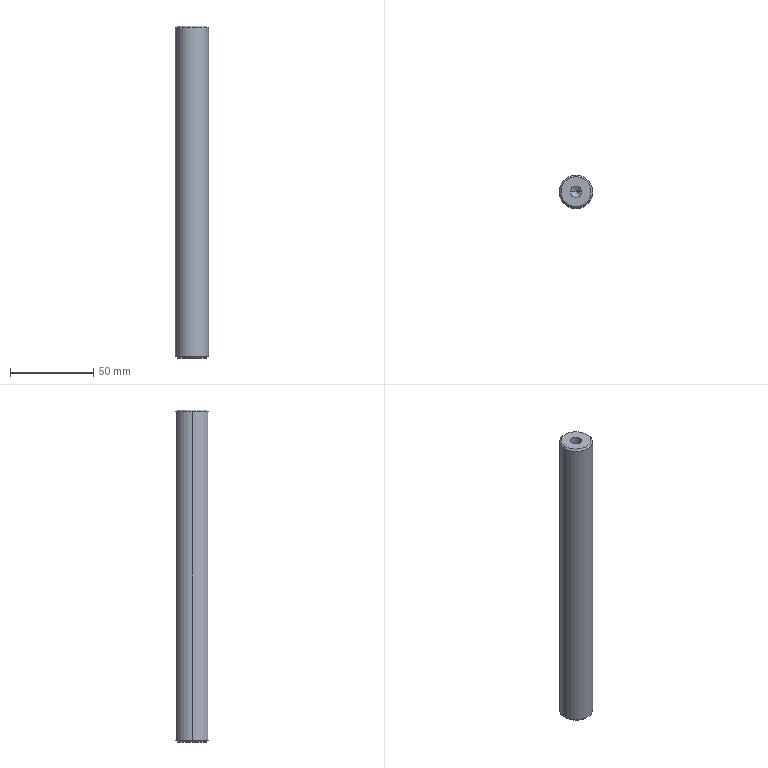Part | SolidWorks | features HoleWzd 2, Chamfer 1, Extrusion 1 | 1 solid | 16 faces | box 20 x 20 x 200 mm | volume 61287 mm3 | cone 8 | cylinder 6 | plane 2 | commonest cylinder face diameters 6.8 x4 20 x2
STEP:
#1=CARTESIAN_POINT('',(9.,0.,200.));
#2=VERTEX_POINT('',#1);
#3=CARTESIAN_POINT('',(-9.,0.,200.));
#4=VERTEX_POINT('',#3);
#5=CARTESIAN_POINT('',(0.,0.,200.));
#6=DIRECTION('',(0.,0.,1.));
#7=DIRECTION('',(1.,0.,0.));
#8=AXIS2_PLACEMENT_3D('',#5,#6,#7);
#9=CIRCLE('',#8,9.);
#10=EDGE_CURVE('',#2,#4,#9,.T.);
#11=ORIENTED_EDGE('',*,*,#10,.F.);
#12=CARTESIAN_POINT('',(10.,0.,199.));
#13=VERTEX_POINT('',#12);
#14=CARTESIAN_POINT('',(9.,0.,200.));
#15=DIRECTION('',(0.7071,0.,-0.7071));
#16=VECTOR('',#15,1000.);
#17=LINE('',#14,#16);
#18=EDGE_CURVE('',#2,#13,#17,.T.);
#19=ORIENTED_EDGE('',*,*,#18,.T.);
#20=CARTESIAN_POINT('',(-10.,0.,199.));
#21=VERTEX_POINT('',#20);
#22=CARTESIAN_POINT('',(0.,0.,199.));
#23=DIRECTION('',(0.,0.,-1.));
#24=DIRECTION('',(1.,0.,0.));
#25=AXIS2_PLACEMENT_3D('',#22,#23,#24);
#26=CIRCLE('',#25,10.);
#27=EDGE_CURVE('',#21,#13,#26,.T.);
#28=ORIENTED_EDGE('',*,*,#27,.F.);
#29=CARTESIAN_POINT('',(-9.,0.,200.));
#30=DIRECTION('',(-0.7071,0.,-0.7071));
#31=VECTOR('',#30,1000.);
#32=LINE('',#29,#31);
#33=EDGE_CURVE('',#4,#21,#32,.T.);
#34=ORIENTED_EDGE('',*,*,#33,.F.);
#35=EDGE_LOOP('',(#11,#19,#28,#34));
#36=FACE_OUTER_BOUND('',#35,.T.);
#37=CARTESIAN_POINT('',(0.,0.,200.));
#38=DIRECTION('',(0.,0.,-1.));
#39=DIRECTION('',(-1.,0.,0.));
#40=AXIS2_PLACEMENT_3D('',#37,#38,#39);
#41=CONICAL_SURFACE('',#40,9.,0.7854);
#42=ADVANCED_FACE('',(#36),#41,.T.);
#43=CARTESIAN_POINT('',(-9.,0.,0.));
#44=VERTEX_POINT('',#43);
#45=CARTESIAN_POINT('',(9.,0.,0.));
#46=VERTEX_POINT('',#45);
#47=CARTESIAN_POINT('',(0.,0.,0.));
#48=DIRECTION('',(0.,0.,-1.));
#49=DIRECTION('',(1.,0.,0.));
#50=AXIS2_PLACEMENT_3D('',#47,#48,#49);
#51=CIRCLE('',#50,9.);
#52=EDGE_CURVE('',#44,#46,#51,.T.);
#53=ORIENTED_EDGE('',*,*,#52,.F.);
#54=CARTESIAN_POINT('',(-10.,0.,1.));
#55=VERTEX_POINT('',#54);
#56=CARTESIAN_POINT('',(-10.,0.,1.));
#57=DIRECTION('',(-0.7071,0.,0.7071));
#58=VECTOR('',#57,1000.);
#59=LINE('',#56,#58);
#60=EDGE_CURVE('',#44,#55,#59,.T.);
#61=ORIENTED_EDGE('',*,*,#60,.T.);
#62=CARTESIAN_POINT('',(10.,0.,1.));
#63=VERTEX_POINT('',#62);
#64=CARTESIAN_POINT('',(0.,0.,1.));
#65=DIRECTION('',(0.,0.,1.));
#66=DIRECTION('',(1.,0.,0.));
#67=AXIS2_PLACEMENT_3D('',#64,#65,#66);
#68=CIRCLE('',#67,10.);
#69=EDGE_CURVE('',#63,#55,#68,.T.);
#70=ORIENTED_EDGE('',*,*,#69,.F.);
#71=CARTESIAN_POINT('',(10.,0.,1.));
#72=DIRECTION('',(0.7071,0.,0.7071));
#73=VECTOR('',#72,1000.);
#74=LINE('',#71,#73);
#75=EDGE_CURVE('',#46,#63,#74,.T.);
#76=ORIENTED_EDGE('',*,*,#75,.F.);
#77=EDGE_LOOP('',(#53,#61,#70,#76));
#78=FACE_OUTER_BOUND('',#77,.T.);
#79=CARTESIAN_POINT('',(0.,0.,1.));
#80=DIRECTION('',(0.,0.,1.));
#81=DIRECTION('',(1.,0.,0.));
#82=AXIS2_PLACEMENT_3D('',#79,#80,#81);
#83=CONICAL_SURFACE('',#82,10.,0.7854);
#84=ADVANCED_FACE('',(#78),#83,.T.);
#85=CARTESIAN_POINT('',(-3.4,0.,180.25));
#86=VERTEX_POINT('',#85);
#87=CARTESIAN_POINT('',(3.4,0.,180.25));
#88=VERTEX_POINT('',#87);
#89=CARTESIAN_POINT('',(0.,0.,180.25));
#90=DIRECTION('',(0.,0.,1.));
#91=DIRECTION('',(1.,0.,0.));
#92=AXIS2_PLACEMENT_3D('',#89,#90,#91);
#93=CIRCLE('',#92,3.4);
#94=EDGE_CURVE('',#86,#88,#93,.T.);
#95=ORIENTED_EDGE('',*,*,#94,.F.);
#96=CARTESIAN_POINT('',(-3.4,0.,200.));
#97=VERTEX_POINT('',#96);
#98=CARTESIAN_POINT('',(-3.4,0.,200.));
#99=DIRECTION('',(0.,0.,1.));
#100=VECTOR('',#99,1000.);
#101=LINE('',#98,#100);
#102=EDGE_CURVE('',#86,#97,#101,.T.);
#103=ORIENTED_EDGE('',*,*,#102,.T.);
#104=CARTESIAN_POINT('',(3.4,0.,200.));
#105=VERTEX_POINT('',#104);
#106=CARTESIAN_POINT('',(0.,0.,200.));
#107=DIRECTION('',(0.,0.,1.));
#108=DIRECTION('',(1.,0.,0.));
#109=AXIS2_PLACEMENT_3D('',#106,#107,#108);
#110=CIRCLE('',#109,3.4);
#111=EDGE_CURVE('',#97,#105,#110,.T.);
#112=ORIENTED_EDGE('',*,*,#111,.T.);
#113=CARTESIAN_POINT('',(3.4,0.,200.));
#114=DIRECTION('',(0.,0.,1.));
#115=VECTOR('',#114,1000.);
#116=LINE('',#113,#115);
#117=EDGE_CURVE('',#88,#105,#116,.T.);
#118=ORIENTED_EDGE('',*,*,#117,.F.);
#119=EDGE_LOOP('',(#95,#103,#112,#118));
#120=FACE_OUTER_BOUND('',#119,.T.);
#121=CARTESIAN_POINT('',(0.,0.,200.));
#122=DIRECTION('',(0.,0.,1.));
#123=DIRECTION('',(1.,0.,0.));
#124=AXIS2_PLACEMENT_3D('',#121,#122,#123);
#125=CYLINDRICAL_SURFACE('',#124,3.4);
#126=ADVANCED_FACE('',(#120),#125,.F.);
#127=CARTESIAN_POINT('',(0.,0.,178.207));
#128=VERTEX_POINT('',#127);
#129=CARTESIAN_POINT('',(3.4,0.,180.25));
#130=DIRECTION('',(0.8572,0.,0.515));
#131=VECTOR('',#130,1000.);
#132=LINE('',#129,#131);
#133=EDGE_CURVE('',#128,#88,#132,.T.);
#134=ORIENTED_EDGE('',*,*,#133,.F.);
#135=CARTESIAN_POINT('',(-3.4,0.,180.25));
#136=DIRECTION('',(-0.8572,0.,0.515));
#137=VECTOR('',#136,1000.);
#138=LINE('',#135,#137);
#139=EDGE_CURVE('',#128,#86,#138,.T.);
#140=ORIENTED_EDGE('',*,*,#139,.T.);
#141=ORIENTED_EDGE('',*,*,#94,.T.);
#142=EDGE_LOOP('',(#134,#140,#141));
#143=FACE_OUTER_BOUND('',#142,.T.);
#144=CARTESIAN_POINT('',(0.,0.,180.25));
#145=DIRECTION('',(0.,0.,1.));
#146=DIRECTION('',(1.,0.,0.));
#147=AXIS2_PLACEMENT_3D('',#144,#145,#146);
#148=CONICAL_SURFACE('',#147,3.4,1.03);
#149=ADVANCED_FACE('',(#143),#148,.F.);
#150=CARTESIAN_POINT('',(3.4,0.,19.75));
#151=VERTEX_POINT('',#150);
#152=CARTESIAN_POINT('',(-3.4,0.,19.75));
#153=VERTEX_POINT('',#152);
#154=CARTESIAN_POINT('',(0.,0.,19.75));
#155=DIRECTION('',(0.,0.,-1.));
#156=DIRECTION('',(-1.,0.,0.));
#157=AXIS2_PLACEMENT_3D('',#154,#155,#156);
#158=CIRCLE('',#157,3.4);
#159=EDGE_CURVE('',#151,#153,#158,.T.);
#160=ORIENTED_EDGE('',*,*,#159,.F.);
#161=CARTESIAN_POINT('',(3.4,0.,0.));
#162=VERTEX_POINT('',#161);
#163=CARTESIAN_POINT('',(3.4,0.,0.));
#164=DIRECTION('',(0.,0.,-1.));
#165=VECTOR('',#164,1000.);
#166=LINE('',#163,#165);
#167=EDGE_CURVE('',#151,#162,#166,.T.);
#168=ORIENTED_EDGE('',*,*,#167,.T.);
#169=CARTESIAN_POINT('',(-3.4,0.,0.));
#170=VERTEX_POINT('',#169);
#171=CARTESIAN_POINT('',(0.,0.,0.));
#172=DIRECTION('',(0.,0.,-1.));
#173=DIRECTION('',(-1.,0.,0.));
#174=AXIS2_PLACEMENT_3D('',#171,#172,#173);
#175=CIRCLE('',#174,3.4);
#176=EDGE_CURVE('',#162,#170,#175,.T.);
#177=ORIENTED_EDGE('',*,*,#176,.T.);
#178=CARTESIAN_POINT('',(-3.4,0.,0.));
#179=DIRECTION('',(0.,0.,-1.));
#180=VECTOR('',#179,1000.);
#181=LINE('',#178,#180);
#182=EDGE_CURVE('',#153,#170,#181,.T.);
#183=ORIENTED_EDGE('',*,*,#182,.F.);
#184=EDGE_LOOP('',(#160,#168,#177,#183));
#185=FACE_OUTER_BOUND('',#184,.T.);
#186=CARTESIAN_POINT('',(0.,0.,0.));
#187=DIRECTION('',(0.,0.,-1.));
#188=DIRECTION('',(-1.,0.,0.));
#189=AXIS2_PLACEMENT_3D('',#186,#187,#188);
#190=CYLINDRICAL_SURFACE('',#189,3.4);
#191=ADVANCED_FACE('',(#185),#190,.F.);
#192=CARTESIAN_POINT('',(0.,0.,21.793));
#193=VERTEX_POINT('',#192);
#194=CARTESIAN_POINT('',(-3.4,0.,19.75));
#195=DIRECTION('',(-0.8572,0.,-0.515));
#196=VECTOR('',#195,1000.);
#197=LINE('',#194,#196);
#198=EDGE_CURVE('',#193,#153,#197,.T.);
#199=ORIENTED_EDGE('',*,*,#198,.F.);
#200=CARTESIAN_POINT('',(3.4,0.,19.75));
#201=DIRECTION('',(0.8572,0.,-0.515));
#202=VECTOR('',#201,1000.);
#203=LINE('',#200,#202);
#204=EDGE_CURVE('',#193,#151,#203,.T.);
#205=ORIENTED_EDGE('',*,*,#204,.T.);
#206=ORIENTED_EDGE('',*,*,#159,.T.);
#207=EDGE_LOOP('',(#199,#205,#206));
#208=FACE_OUTER_BOUND('',#207,.T.);
#209=CARTESIAN_POINT('',(0.,0.,19.75));
#210=DIRECTION('',(0.,0.,-1.));
#211=DIRECTION('',(-1.,0.,0.));
#212=AXIS2_PLACEMENT_3D('',#209,#210,#211);
#213=CONICAL_SURFACE('',#212,3.4,1.03);
#214=ADVANCED_FACE('',(#208),#213,.F.);
#215=ORIENTED_EDGE('',*,*,#27,.T.);
#216=CARTESIAN_POINT('',(10.,0.,200.));
#217=DIRECTION('',(0.,0.,-1.));
#218=VECTOR('',#217,1000.);
#219=LINE('',#216,#218);
#220=EDGE_CURVE('',#13,#63,#219,.T.);
#221=ORIENTED_EDGE('',*,*,#220,.T.);
#222=ORIENTED_EDGE('',*,*,#69,.T.);
#223=CARTESIAN_POINT('',(-10.,0.,200.));
#224=DIRECTION('',(0.,0.,-1.));
#225=VECTOR('',#224,1000.);
#226=LINE('',#223,#225);
#227=EDGE_CURVE('',#21,#55,#226,.T.);
#228=ORIENTED_EDGE('',*,*,#227,.F.);
#229=EDGE_LOOP('',(#215,#221,#222,#228));
#230=FACE_OUTER_BOUND('',#229,.T.);
#231=CARTESIAN_POINT('',(0.,0.,200.));
#232=DIRECTION('',(0.,0.,-1.));
#233=DIRECTION('',(-1.,0.,0.));
#234=AXIS2_PLACEMENT_3D('',#231,#232,#233);
#235=CYLINDRICAL_SURFACE('',#234,10.);
#236=ADVANCED_FACE('',(#230),#235,.T.);
#237=ORIENTED_EDGE('',*,*,#220,.F.);
#238=CARTESIAN_POINT('',(0.,0.,199.));
#239=DIRECTION('',(0.,0.,-1.));
#240=DIRECTION('',(1.,0.,0.));
#241=AXIS2_PLACEMENT_3D('',#238,#239,#240);
#242=CIRCLE('',#241,10.);
#243=EDGE_CURVE('',#13,#21,#242,.T.);
#244=ORIENTED_EDGE('',*,*,#243,.T.);
#245=ORIENTED_EDGE('',*,*,#227,.T.);
#246=CARTESIAN_POINT('',(0.,0.,1.));
#247=DIRECTION('',(0.,0.,1.));
#248=DIRECTION('',(1.,0.,0.));
#249=AXIS2_PLACEMENT_3D('',#246,#247,#248);
#250=CIRCLE('',#249,10.);
#251=EDGE_CURVE('',#55,#63,#250,.T.);
#252=ORIENTED_EDGE('',*,*,#251,.T.);
#253=EDGE_LOOP('',(#237,#244,#245,#252));
#254=FACE_OUTER_BOUND('',#253,.T.);
#255=CARTESIAN_POINT('',(0.,0.,200.));
#256=DIRECTION('',(0.,0.,-1.));
#257=DIRECTION('',(-1.,0.,0.));
#258=AXIS2_PLACEMENT_3D('',#255,#256,#257);
#259=CYLINDRICAL_SURFACE('',#258,10.);
#260=ADVANCED_FACE('',(#254),#259,.T.);
#261=CARTESIAN_POINT('',(0.,0.,200.));
#262=DIRECTION('',(0.,0.,1.));
#263=DIRECTION('',(1.,0.,0.));
#264=AXIS2_PLACEMENT_3D('',#261,#262,#263);
#265=CIRCLE('',#264,9.);
#266=EDGE_CURVE('',#4,#2,#265,.T.);
#267=ORIENTED_EDGE('',*,*,#266,.T.);
#268=ORIENTED_EDGE('',*,*,#10,.T.);
#269=EDGE_LOOP('',(#267,#268));
#270=FACE_OUTER_BOUND('',#269,.T.);
#271=CARTESIAN_POINT('',(0.,0.,200.));
#272=DIRECTION('',(0.,0.,1.));
#273=DIRECTION('',(1.,0.,0.));
#274=AXIS2_PLACEMENT_3D('',#271,#272,#273);
#275=CIRCLE('',#274,3.4);
#276=EDGE_CURVE('',#105,#97,#275,.T.);
#277=ORIENTED_EDGE('',*,*,#276,.F.);
#278=ORIENTED_EDGE('',*,*,#111,.F.);
#279=EDGE_LOOP('',(#277,#278));
#280=FACE_BOUND('',#279,.T.);
#281=CARTESIAN_POINT('',(0.,0.,200.));
#282=DIRECTION('',(0.,0.,1.));
#283=DIRECTION('',(1.,0.,0.));
#284=AXIS2_PLACEMENT_3D('',#281,#282,#283);
#285=PLANE('',#284);
#286=ADVANCED_FACE('',(#270,#280),#285,.T.);
#287=CARTESIAN_POINT('',(0.,0.,0.));
#288=DIRECTION('',(0.,0.,-1.));
#289=DIRECTION('',(1.,0.,0.));
#290=AXIS2_PLACEMENT_3D('',#287,#288,#289);
#291=CIRCLE('',#290,9.);
#292=EDGE_CURVE('',#46,#44,#291,.T.);
#293=ORIENTED_EDGE('',*,*,#292,.T.);
#294=ORIENTED_EDGE('',*,*,#52,.T.);
#295=EDGE_LOOP('',(#293,#294));
#296=FACE_OUTER_BOUND('',#295,.T.);
#297=CARTESIAN_POINT('',(0.,0.,0.));
#298=DIRECTION('',(0.,0.,-1.));
#299=DIRECTION('',(-1.,0.,0.));
#300=AXIS2_PLACEMENT_3D('',#297,#298,#299);
#301=CIRCLE('',#300,3.4);
#302=EDGE_CURVE('',#170,#162,#301,.T.);
#303=ORIENTED_EDGE('',*,*,#302,.F.);
#304=ORIENTED_EDGE('',*,*,#176,.F.);
#305=EDGE_LOOP('',(#303,#304));
#306=FACE_BOUND('',#305,.T.);
#307=CARTESIAN_POINT('',(0.,0.,0.));
#308=DIRECTION('',(0.,0.,1.));
#309=DIRECTION('',(1.,0.,0.));
#310=AXIS2_PLACEMENT_3D('',#307,#308,#309);
#311=PLANE('',#310);
#312=ADVANCED_FACE('',(#296,#306),#311,.F.);
#313=ORIENTED_EDGE('',*,*,#204,.F.);
#314=ORIENTED_EDGE('',*,*,#198,.T.);
#315=CARTESIAN_POINT('',(0.,0.,19.75));
#316=DIRECTION('',(0.,0.,-1.));
#317=DIRECTION('',(-1.,0.,0.));
#318=AXIS2_PLACEMENT_3D('',#315,#316,#317);
#319=CIRCLE('',#318,3.4);
#320=EDGE_CURVE('',#153,#151,#319,.T.);
#321=ORIENTED_EDGE('',*,*,#320,.T.);
#322=EDGE_LOOP('',(#313,#314,#321));
#323=FACE_OUTER_BOUND('',#322,.T.);
#324=CARTESIAN_POINT('',(0.,0.,19.75));
#325=DIRECTION('',(0.,0.,-1.));
#326=DIRECTION('',(-1.,0.,0.));
#327=AXIS2_PLACEMENT_3D('',#324,#325,#326);
#328=CONICAL_SURFACE('',#327,3.4,1.03);
#329=ADVANCED_FACE('',(#323),#328,.F.);
#330=ORIENTED_EDGE('',*,*,#167,.F.);
#331=ORIENTED_EDGE('',*,*,#320,.F.);
#332=ORIENTED_EDGE('',*,*,#182,.T.);
#333=ORIENTED_EDGE('',*,*,#302,.T.);
#334=EDGE_LOOP('',(#330,#331,#332,#333));
#335=FACE_OUTER_BOUND('',#334,.T.);
#336=CARTESIAN_POINT('',(0.,0.,0.));
#337=DIRECTION('',(0.,0.,-1.));
#338=DIRECTION('',(-1.,0.,0.));
#339=AXIS2_PLACEMENT_3D('',#336,#337,#338);
#340=CYLINDRICAL_SURFACE('',#339,3.4);
#341=ADVANCED_FACE('',(#335),#340,.F.);
#342=ORIENTED_EDGE('',*,*,#139,.F.);
#343=ORIENTED_EDGE('',*,*,#133,.T.);
#344=CARTESIAN_POINT('',(0.,0.,180.25));
#345=DIRECTION('',(0.,0.,1.));
#346=DIRECTION('',(1.,0.,0.));
#347=AXIS2_PLACEMENT_3D('',#344,#345,#346);
#348=CIRCLE('',#347,3.4);
#349=EDGE_CURVE('',#88,#86,#348,.T.);
#350=ORIENTED_EDGE('',*,*,#349,.T.);
#351=EDGE_LOOP('',(#342,#343,#350));
#352=FACE_OUTER_BOUND('',#351,.T.);
#353=CARTESIAN_POINT('',(0.,0.,180.25));
#354=DIRECTION('',(0.,0.,1.));
#355=DIRECTION('',(1.,0.,0.));
#356=AXIS2_PLACEMENT_3D('',#353,#354,#355);
#357=CONICAL_SURFACE('',#356,3.4,1.03);
#358=ADVANCED_FACE('',(#352),#357,.F.);
#359=ORIENTED_EDGE('',*,*,#102,.F.);
#360=ORIENTED_EDGE('',*,*,#349,.F.);
#361=ORIENTED_EDGE('',*,*,#117,.T.);
#362=ORIENTED_EDGE('',*,*,#276,.T.);
#363=EDGE_LOOP('',(#359,#360,#361,#362));
#364=FACE_OUTER_BOUND('',#363,.T.);
#365=CARTESIAN_POINT('',(0.,0.,200.));
#366=DIRECTION('',(0.,0.,1.));
#367=DIRECTION('',(1.,0.,0.));
#368=AXIS2_PLACEMENT_3D('',#365,#366,#367);
#369=CYLINDRICAL_SURFACE('',#368,3.4);
#370=ADVANCED_FACE('',(#364),#369,.F.);
#371=ORIENTED_EDGE('',*,*,#60,.F.);
#372=ORIENTED_EDGE('',*,*,#292,.F.);
#373=ORIENTED_EDGE('',*,*,#75,.T.);
#374=ORIENTED_EDGE('',*,*,#251,.F.);
#375=EDGE_LOOP('',(#371,#372,#373,#374));
#376=FACE_OUTER_BOUND('',#375,.T.);
#377=CARTESIAN_POINT('',(0.,0.,1.));
#378=DIRECTION('',(0.,0.,1.));
#379=DIRECTION('',(1.,0.,0.));
#380=AXIS2_PLACEMENT_3D('',#377,#378,#379);
#381=CONICAL_SURFACE('',#380,10.,0.7854);
#382=ADVANCED_FACE('',(#376),#381,.T.);
#383=ORIENTED_EDGE('',*,*,#18,.F.);
#384=ORIENTED_EDGE('',*,*,#266,.F.);
#385=ORIENTED_EDGE('',*,*,#33,.T.);
#386=ORIENTED_EDGE('',*,*,#243,.F.);
#387=EDGE_LOOP('',(#383,#384,#385,#386));
#388=FACE_OUTER_BOUND('',#387,.T.);
#389=CARTESIAN_POINT('',(0.,0.,200.));
#390=DIRECTION('',(0.,0.,-1.));
#391=DIRECTION('',(-1.,0.,0.));
#392=AXIS2_PLACEMENT_3D('',#389,#390,#391);
#393=CONICAL_SURFACE('',#392,9.,0.7854);
#394=ADVANCED_FACE('',(#388),#393,.T.);
#395=CLOSED_SHELL('',(#42,#84,#126,#149,#191,#214,#236,#260,#286,#312,#329,#341,#358,#370,#382,#394));
#396=MANIFOLD_SOLID_BREP('',#395);
#397=CARTESIAN_POINT('',(0.,0.,0.));
#398=DIRECTION('',(0.,0.,1.));
#399=DIRECTION('',(1.,0.,0.));
#400=AXIS2_PLACEMENT_3D('',#397,#398,#399);
#401=(LENGTH_UNIT()NAMED_UNIT(*)SI_UNIT(.MILLI.,.METRE.));
#402=UNCERTAINTY_MEASURE_WITH_UNIT(LENGTH_MEASURE(0.00001),#401,'','');
#403=(NAMED_UNIT(*)PLANE_ANGLE_UNIT()SI_UNIT($,.RADIAN.));
#404=(NAMED_UNIT(*)SI_UNIT($,.STERADIAN.)SOLID_ANGLE_UNIT());
#405=(GEOMETRIC_REPRESENTATION_CONTEXT(3)GLOBAL_UNCERTAINTY_ASSIGNED_CONTEXT((#402))GLOBAL_UNIT_ASSIGNED_CONTEXT((#401,#403,#404))REPRESENTATION_CONTEXT('',''));
#406=ADVANCED_BREP_SHAPE_REPRESENTATION('',(#396,#400),#405);